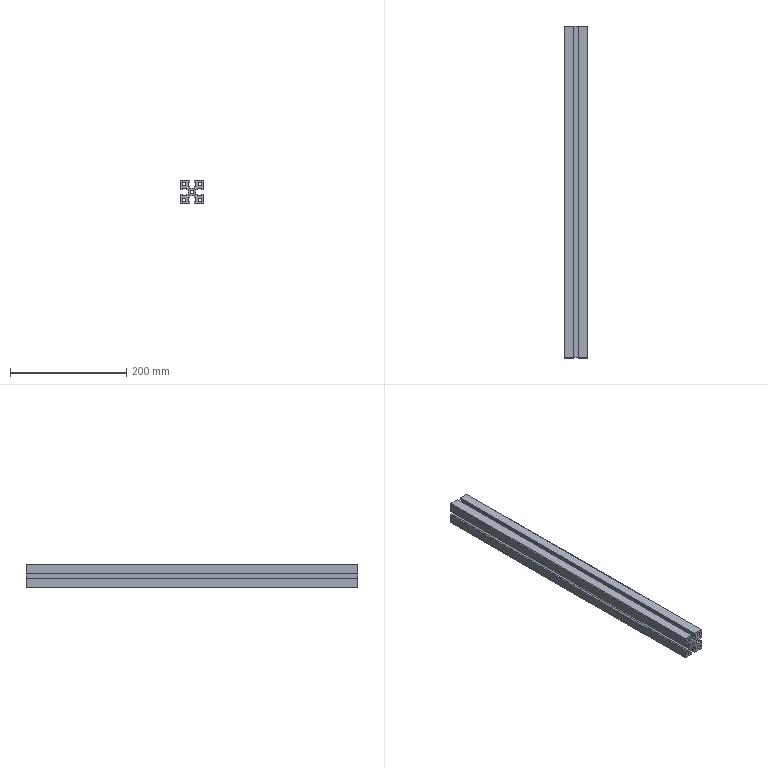Part | STEP file | 01-02 Bracket post 2 | 1 solid | 68 faces | box 40 x 570 x 40 mm | volume 524269 mm3 | plane 54 | cylinder 14 | commonest cylinder face diameters 6 x10 2 x4